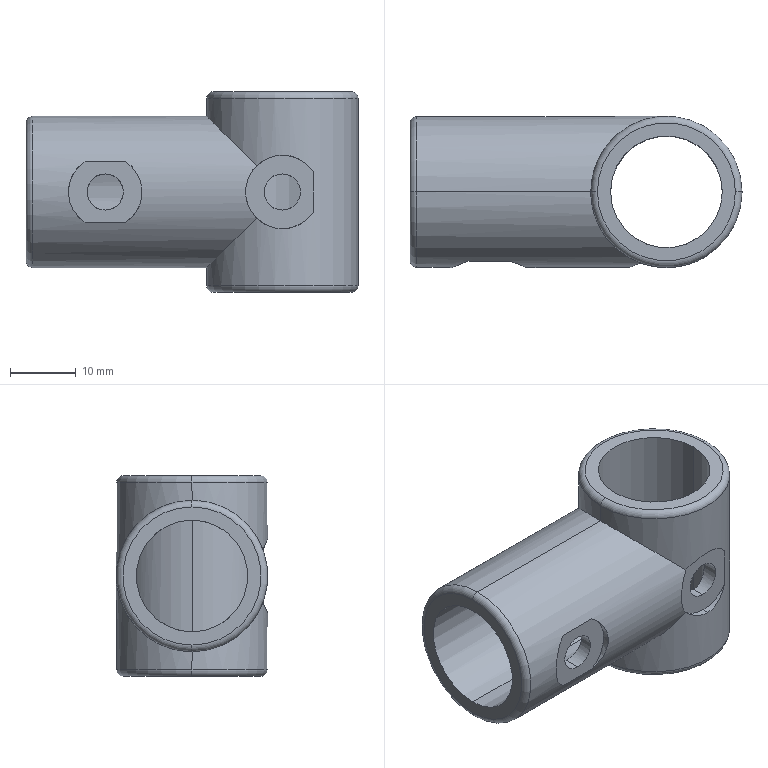Part | SolidWorks | features BaseBody 1 | 1 solid | 30 faces | box 50.5 x 23 x 30.5 mm | volume 11175 mm3 | cylinder 19 | torus 6 | plane 5 | commonest cylinder face diameters 23 x6 11.2 x5 5.5 x4 17 x4
STEP:
#1=CARTESIAN_POINT('',(0.,11.5,15.25));
#2=VERTEX_POINT('',#1);
#3=CARTESIAN_POINT('',(-11.5,0.,3.75));
#4=VERTEX_POINT('',#3);
#5=CARTESIAN_POINT('',(0.,11.5,15.25));
#6=CARTESIAN_POINT('',(-6.737,11.5,8.513));
#7=CARTESIAN_POINT('',(-11.5,6.737,3.75));
#8=CARTESIAN_POINT('',(-11.5,0.,3.75));
#9=(BOUNDED_CURVE()B_SPLINE_CURVE(3,(#5,#6,#7,#8),.UNSPECIFIED.,.F.,.F.)B_SPLINE_CURVE_WITH_KNOTS((4,4),(4.712,6.283),.UNSPECIFIED.)CURVE()GEOMETRIC_REPRESENTATION_ITEM()RATIONAL_B_SPLINE_CURVE((1.,0.8047,0.8047,1.))REPRESENTATION_ITEM(''));
#10=EDGE_CURVE('',#2,#4,#9,.T.);
#11=ORIENTED_EDGE('',*,*,#10,.T.);
#12=CARTESIAN_POINT('',(-38.,0.,3.75));
#13=VERTEX_POINT('',#12);
#14=CARTESIAN_POINT('',(11.501,0.,3.75));
#15=DIRECTION('',(-1.,0.,0.));
#16=VECTOR('',#15,1000.);
#17=LINE('',#14,#16);
#18=EDGE_CURVE('',#4,#13,#17,.T.);
#19=ORIENTED_EDGE('',*,*,#18,.T.);
#20=CARTESIAN_POINT('',(-38.,0.,26.75));
#21=VERTEX_POINT('',#20);
#22=CARTESIAN_POINT('',(-38.,0.,15.25));
#23=DIRECTION('',(1.,0.,0.));
#24=DIRECTION('',(0.,0.,1.));
#25=AXIS2_PLACEMENT_3D('',#22,#23,#24);
#26=CIRCLE('',#25,11.5);
#27=EDGE_CURVE('',#13,#21,#26,.T.);
#28=ORIENTED_EDGE('',*,*,#27,.T.);
#29=CARTESIAN_POINT('',(-11.5,0.,26.75));
#30=VERTEX_POINT('',#29);
#31=CARTESIAN_POINT('',(11.501,0.,26.75));
#32=DIRECTION('',(-1.,0.,0.));
#33=VECTOR('',#32,1000.);
#34=LINE('',#31,#33);
#35=EDGE_CURVE('',#30,#21,#34,.T.);
#36=ORIENTED_EDGE('',*,*,#35,.F.);
#37=CARTESIAN_POINT('',(-11.5,0.,26.75));
#38=CARTESIAN_POINT('',(-11.5,6.737,26.75));
#39=CARTESIAN_POINT('',(-6.737,11.5,21.987));
#40=CARTESIAN_POINT('',(0.,11.5,15.25));
#41=(BOUNDED_CURVE()B_SPLINE_CURVE(3,(#37,#38,#39,#40),.UNSPECIFIED.,.F.,.F.)B_SPLINE_CURVE_WITH_KNOTS((4,4),(3.142,4.712),.UNSPECIFIED.)CURVE()GEOMETRIC_REPRESENTATION_ITEM()RATIONAL_B_SPLINE_CURVE((1.,0.8047,0.8047,1.))REPRESENTATION_ITEM(''));
#42=EDGE_CURVE('',#30,#2,#41,.T.);
#43=ORIENTED_EDGE('',*,*,#42,.T.);
#44=EDGE_LOOP('',(#11,#19,#28,#36,#43));
#45=FACE_OUTER_BOUND('',#44,.T.);
#46=CARTESIAN_POINT('',(11.501,0.,15.25));
#47=DIRECTION('',(-1.,0.,0.));
#48=DIRECTION('',(0.,0.,1.));
#49=AXIS2_PLACEMENT_3D('',#46,#47,#48);
#50=CYLINDRICAL_SURFACE('',#49,11.5);
#51=ADVANCED_FACE('',(#45),#50,.T.);
#52=CARTESIAN_POINT('',(-11.5,0.,29.5));
#53=VERTEX_POINT('',#52);
#54=CARTESIAN_POINT('',(11.5,0.,29.5));
#55=VERTEX_POINT('',#54);
#56=CARTESIAN_POINT('',(0.,0.,29.5));
#57=DIRECTION('',(0.,0.,-1.));
#58=DIRECTION('',(-1.,0.,0.));
#59=AXIS2_PLACEMENT_3D('',#56,#57,#58);
#60=CIRCLE('',#59,11.5);
#61=EDGE_CURVE('',#53,#55,#60,.T.);
#62=ORIENTED_EDGE('',*,*,#61,.T.);
#63=CARTESIAN_POINT('',(11.5,0.,1.));
#64=VERTEX_POINT('',#63);
#65=CARTESIAN_POINT('',(11.5,0.,30.5));
#66=DIRECTION('',(0.,0.,-1.));
#67=VECTOR('',#66,1000.);
#68=LINE('',#65,#67);
#69=EDGE_CURVE('',#55,#64,#68,.T.);
#70=ORIENTED_EDGE('',*,*,#69,.T.);
#71=CARTESIAN_POINT('',(-11.5,0.,1.));
#72=VERTEX_POINT('',#71);
#73=CARTESIAN_POINT('',(0.,0.,1.));
#74=DIRECTION('',(0.,0.,1.));
#75=DIRECTION('',(-1.,0.,0.));
#76=AXIS2_PLACEMENT_3D('',#73,#74,#75);
#77=CIRCLE('',#76,11.5);
#78=EDGE_CURVE('',#64,#72,#77,.T.);
#79=ORIENTED_EDGE('',*,*,#78,.T.);
#80=CARTESIAN_POINT('',(-11.5,0.,30.5));
#81=DIRECTION('',(0.,0.,-1.));
#82=VECTOR('',#81,1000.);
#83=LINE('',#80,#82);
#84=EDGE_CURVE('',#4,#72,#83,.T.);
#85=ORIENTED_EDGE('',*,*,#84,.F.);
#86=ORIENTED_EDGE('',*,*,#10,.F.);
#87=ORIENTED_EDGE('',*,*,#42,.F.);
#88=CARTESIAN_POINT('',(-11.5,0.,30.5));
#89=DIRECTION('',(0.,0.,-1.));
#90=VECTOR('',#89,1000.);
#91=LINE('',#88,#90);
#92=EDGE_CURVE('',#53,#30,#91,.T.);
#93=ORIENTED_EDGE('',*,*,#92,.F.);
#94=EDGE_LOOP('',(#62,#70,#79,#85,#86,#87,#93));
#95=FACE_OUTER_BOUND('',#94,.T.);
#96=CARTESIAN_POINT('',(0.,0.,30.5));
#97=DIRECTION('',(0.,0.,-1.));
#98=DIRECTION('',(-1.,0.,0.));
#99=AXIS2_PLACEMENT_3D('',#96,#97,#98);
#100=CYLINDRICAL_SURFACE('',#99,11.5);
#101=ADVANCED_FACE('',(#95),#100,.T.);
#102=CARTESIAN_POINT('',(-39.,0.,4.75));
#103=VERTEX_POINT('',#102);
#104=CARTESIAN_POINT('',(-39.,0.,25.75));
#105=VERTEX_POINT('',#104);
#106=CARTESIAN_POINT('',(-39.,0.,15.25));
#107=DIRECTION('',(1.,0.,0.));
#108=DIRECTION('',(0.,0.,-1.));
#109=AXIS2_PLACEMENT_3D('',#106,#107,#108);
#110=CIRCLE('',#109,10.5);
#111=EDGE_CURVE('',#103,#105,#110,.T.);
#112=ORIENTED_EDGE('',*,*,#111,.T.);
#113=CARTESIAN_POINT('',(-38.,0.,25.75));
#114=DIRECTION('',(0.,1.,0.));
#115=DIRECTION('',(0.,0.,1.));
#116=AXIS2_PLACEMENT_3D('',#113,#114,#115);
#117=CIRCLE('',#116,1.);
#118=EDGE_CURVE('',#105,#21,#117,.T.);
#119=ORIENTED_EDGE('',*,*,#118,.T.);
#120=ORIENTED_EDGE('',*,*,#27,.F.);
#121=CARTESIAN_POINT('',(-38.,0.,4.75));
#122=DIRECTION('',(0.,-1.,0.));
#123=DIRECTION('',(0.,0.,-1.));
#124=AXIS2_PLACEMENT_3D('',#121,#122,#123);
#125=CIRCLE('',#124,1.);
#126=EDGE_CURVE('',#103,#13,#125,.T.);
#127=ORIENTED_EDGE('',*,*,#126,.F.);
#128=EDGE_LOOP('',(#112,#119,#120,#127));
#129=FACE_OUTER_BOUND('',#128,.T.);
#130=CARTESIAN_POINT('',(-38.,0.,15.25));
#131=DIRECTION('',(1.,0.,0.));
#132=DIRECTION('',(0.,0.,-1.));
#133=AXIS2_PLACEMENT_3D('',#130,#131,#132);
#134=TOROIDAL_SURFACE('',#133,10.5,1.);
#135=ADVANCED_FACE('',(#129),#134,.T.);
#136=CARTESIAN_POINT('',(10.5,0.,0.));
#137=VERTEX_POINT('',#136);
#138=CARTESIAN_POINT('',(-10.5,0.,0.));
#139=VERTEX_POINT('',#138);
#140=CARTESIAN_POINT('',(0.,0.,0.));
#141=DIRECTION('',(0.,0.,1.));
#142=DIRECTION('',(1.,0.,0.));
#143=AXIS2_PLACEMENT_3D('',#140,#141,#142);
#144=CIRCLE('',#143,10.5);
#145=EDGE_CURVE('',#137,#139,#144,.T.);
#146=ORIENTED_EDGE('',*,*,#145,.T.);
#147=CARTESIAN_POINT('',(-10.5,0.,1.));
#148=DIRECTION('',(0.,1.,0.));
#149=DIRECTION('',(-1.,0.,0.));
#150=AXIS2_PLACEMENT_3D('',#147,#148,#149);
#151=CIRCLE('',#150,1.);
#152=EDGE_CURVE('',#139,#72,#151,.T.);
#153=ORIENTED_EDGE('',*,*,#152,.T.);
#154=ORIENTED_EDGE('',*,*,#78,.F.);
#155=CARTESIAN_POINT('',(10.5,0.,1.));
#156=DIRECTION('',(0.,-1.,0.));
#157=DIRECTION('',(0.,0.,-1.));
#158=AXIS2_PLACEMENT_3D('',#155,#156,#157);
#159=CIRCLE('',#158,1.);
#160=EDGE_CURVE('',#137,#64,#159,.T.);
#161=ORIENTED_EDGE('',*,*,#160,.F.);
#162=EDGE_LOOP('',(#146,#153,#154,#161));
#163=FACE_OUTER_BOUND('',#162,.T.);
#164=CARTESIAN_POINT('',(0.,0.,1.));
#165=DIRECTION('',(0.,0.,1.));
#166=DIRECTION('',(1.,0.,0.));
#167=AXIS2_PLACEMENT_3D('',#164,#165,#166);
#168=TOROIDAL_SURFACE('',#167,10.5,1.);
#169=ADVANCED_FACE('',(#163),#168,.T.);
#170=ORIENTED_EDGE('',*,*,#61,.F.);
#171=CARTESIAN_POINT('',(-10.5,0.,30.5));
#172=VERTEX_POINT('',#171);
#173=CARTESIAN_POINT('',(-10.5,0.,29.5));
#174=DIRECTION('',(0.,1.,0.));
#175=DIRECTION('',(-1.,0.,0.));
#176=AXIS2_PLACEMENT_3D('',#173,#174,#175);
#177=CIRCLE('',#176,1.);
#178=EDGE_CURVE('',#53,#172,#177,.T.);
#179=ORIENTED_EDGE('',*,*,#178,.T.);
#180=CARTESIAN_POINT('',(10.5,0.,30.5));
#181=VERTEX_POINT('',#180);
#182=CARTESIAN_POINT('',(0.,0.,30.5));
#183=DIRECTION('',(0.,0.,-1.));
#184=DIRECTION('',(1.,0.,0.));
#185=AXIS2_PLACEMENT_3D('',#182,#183,#184);
#186=CIRCLE('',#185,10.5);
#187=EDGE_CURVE('',#172,#181,#186,.T.);
#188=ORIENTED_EDGE('',*,*,#187,.T.);
#189=CARTESIAN_POINT('',(10.5,0.,29.5));
#190=DIRECTION('',(0.,-1.,0.));
#191=DIRECTION('',(0.,0.,-1.));
#192=AXIS2_PLACEMENT_3D('',#189,#190,#191);
#193=CIRCLE('',#192,1.);
#194=EDGE_CURVE('',#55,#181,#193,.T.);
#195=ORIENTED_EDGE('',*,*,#194,.F.);
#196=EDGE_LOOP('',(#170,#179,#188,#195));
#197=FACE_OUTER_BOUND('',#196,.T.);
#198=CARTESIAN_POINT('',(0.,0.,29.5));
#199=DIRECTION('',(0.,0.,1.));
#200=DIRECTION('',(1.,0.,0.));
#201=AXIS2_PLACEMENT_3D('',#198,#199,#200);
#202=TOROIDAL_SURFACE('',#201,10.5,1.);
#203=ADVANCED_FACE('',(#197),#202,.T.);
#204=CARTESIAN_POINT('',(0.,-10.5,20.85));
#205=VERTEX_POINT('',#204);
#206=CARTESIAN_POINT('',(0.,-10.5,9.65));
#207=VERTEX_POINT('',#206);
#208=CARTESIAN_POINT('',(0.,-10.5,15.25));
#209=DIRECTION('',(0.,-1.,0.));
#210=DIRECTION('',(0.,0.,-1.));
#211=AXIS2_PLACEMENT_3D('',#208,#209,#210);
#212=CIRCLE('',#211,5.6);
#213=EDGE_CURVE('',#205,#207,#212,.T.);
#214=ORIENTED_EDGE('',*,*,#213,.F.);
#215=CARTESIAN_POINT('',(0.,-11.5,20.85));
#216=VERTEX_POINT('',#215);
#217=CARTESIAN_POINT('',(0.,-10.5,20.85));
#218=DIRECTION('',(0.,-1.,0.));
#219=VECTOR('',#218,1000.);
#220=LINE('',#217,#219);
#221=EDGE_CURVE('',#205,#216,#220,.T.);
#222=ORIENTED_EDGE('',*,*,#221,.T.);
#223=CARTESIAN_POINT('',(-3.96,-10.797,19.21));
#224=VERTEX_POINT('',#223);
#225=CARTESIAN_POINT('',(-3.96,-10.797,19.21));
#226=CARTESIAN_POINT('',(-3.703,-10.891,19.467));
#227=CARTESIAN_POINT('',(-3.425,-10.983,19.695));
#228=CARTESIAN_POINT('',(-2.976,-11.109,19.997));
#229=CARTESIAN_POINT('',(-2.821,-11.15,20.091));
#230=CARTESIAN_POINT('',(-2.5,-11.226,20.264));
#231=CARTESIAN_POINT('',(-2.333,-11.262,20.344));
#232=CARTESIAN_POINT('',(-1.826,-11.359,20.557));
#233=CARTESIAN_POINT('',(-1.476,-11.411,20.665));
#234=CARTESIAN_POINT('',(-0.7521,-11.481,20.812));
#235=CARTESIAN_POINT('',(-0.3759,-11.5,20.85));
#236=CARTESIAN_POINT('',(0.,-11.5,20.85));
#237=B_SPLINE_CURVE_WITH_KNOTS('',3,(#225,#226,#227,#228,#229,#230,#231,#232,#233,#234,#235,#236),.UNSPECIFIED.,.F.,.F.,(4,2,2,2,2,4),(-0.004442,-0.003332,-0.002776,-0.002221,-0.001111,0.),.UNSPECIFIED.);
#238=EDGE_CURVE('',#224,#216,#237,.T.);
#239=ORIENTED_EDGE('',*,*,#238,.F.);
#240=CARTESIAN_POINT('',(-3.96,-10.797,11.29));
#241=VERTEX_POINT('',#240);
#242=CARTESIAN_POINT('',(-3.96,-10.797,11.29));
#243=CARTESIAN_POINT('',(-4.217,-10.891,11.547));
#244=CARTESIAN_POINT('',(-4.445,-10.983,11.825));
#245=CARTESIAN_POINT('',(-4.747,-11.109,12.274));
#246=CARTESIAN_POINT('',(-4.841,-11.15,12.429));
#247=CARTESIAN_POINT('',(-5.015,-11.226,12.751));
#248=CARTESIAN_POINT('',(-5.094,-11.262,12.918));
#249=CARTESIAN_POINT('',(-5.307,-11.359,13.425));
#250=CARTESIAN_POINT('',(-5.415,-11.411,13.775));
#251=CARTESIAN_POINT('',(-5.562,-11.481,14.499));
#252=CARTESIAN_POINT('',(-5.6,-11.5,14.876));
#253=CARTESIAN_POINT('',(-5.6,-11.5,15.617));
#254=CARTESIAN_POINT('',(-5.564,-11.482,15.986));
#255=CARTESIAN_POINT('',(-5.417,-11.412,16.719));
#256=CARTESIAN_POINT('',(-5.308,-11.36,17.071));
#257=CARTESIAN_POINT('',(-5.026,-11.231,17.746));
#258=CARTESIAN_POINT('',(-4.85,-11.153,18.072));
#259=CARTESIAN_POINT('',(-4.446,-10.983,18.674));
#260=CARTESIAN_POINT('',(-4.217,-10.891,18.953));
#261=CARTESIAN_POINT('',(-3.96,-10.797,19.21));
#262=B_SPLINE_CURVE_WITH_KNOTS('',3,(#242,#243,#244,#245,#246,#247,#248,#249,#250,#251,#252,#253,#254,#255,#256,#257,#258,#259,#260,#261),.UNSPECIFIED.,.F.,.F.,(4,2,2,2,2,2,2,2,2,4),(0.,0.001111,0.001667,0.002222,0.003334,0.004445,0.005556,0.006667,0.007779,0.00889),.UNSPECIFIED.);
#263=EDGE_CURVE('',#241,#224,#262,.T.);
#264=ORIENTED_EDGE('',*,*,#263,.F.);
#265=CARTESIAN_POINT('',(0.,-11.5,9.65));
#266=VERTEX_POINT('',#265);
#267=CARTESIAN_POINT('',(0.,-11.5,9.65));
#268=CARTESIAN_POINT('',(-0.3755,-11.5,9.65));
#269=CARTESIAN_POINT('',(-0.7436,-11.482,9.687));
#270=CARTESIAN_POINT('',(-1.466,-11.412,9.833));
#271=CARTESIAN_POINT('',(-1.824,-11.36,9.943));
#272=CARTESIAN_POINT('',(-2.499,-11.23,10.225));
#273=CARTESIAN_POINT('',(-2.818,-11.154,10.397));
#274=CARTESIAN_POINT('',(-3.422,-10.984,10.802));
#275=CARTESIAN_POINT('',(-3.703,-10.891,11.034));
#276=CARTESIAN_POINT('',(-3.96,-10.797,11.29));
#277=B_SPLINE_CURVE_WITH_KNOTS('',3,(#267,#268,#269,#270,#271,#272,#273,#274,#275,#276),.UNSPECIFIED.,.F.,.F.,(4,2,2,2,4),(0.,0.001109,0.002219,0.003328,0.004437),.UNSPECIFIED.);
#278=EDGE_CURVE('',#266,#241,#277,.T.);
#279=ORIENTED_EDGE('',*,*,#278,.F.);
#280=CARTESIAN_POINT('',(0.,-10.5,9.65));
#281=DIRECTION('',(0.,-1.,0.));
#282=VECTOR('',#281,1000.);
#283=LINE('',#280,#282);
#284=EDGE_CURVE('',#207,#266,#283,.T.);
#285=ORIENTED_EDGE('',*,*,#284,.F.);
#286=EDGE_LOOP('',(#214,#222,#239,#264,#279,#285));
#287=FACE_OUTER_BOUND('',#286,.T.);
#288=CARTESIAN_POINT('',(0.,-10.5,15.25));
#289=DIRECTION('',(0.,-1.,0.));
#290=DIRECTION('',(0.,0.,-1.));
#291=AXIS2_PLACEMENT_3D('',#288,#289,#290);
#292=CYLINDRICAL_SURFACE('',#291,5.6);
#293=ADVANCED_FACE('',(#287),#292,.F.);
#294=CARTESIAN_POINT('',(4.69,-10.5,12.191));
#295=VERTEX_POINT('',#294);
#296=CARTESIAN_POINT('',(0.,-10.5,15.25));
#297=DIRECTION('',(0.,-1.,0.));
#298=DIRECTION('',(0.,0.,-1.));
#299=AXIS2_PLACEMENT_3D('',#296,#297,#298);
#300=CIRCLE('',#299,5.6);
#301=EDGE_CURVE('',#207,#295,#300,.T.);
#302=ORIENTED_EDGE('',*,*,#301,.F.);
#303=ORIENTED_EDGE('',*,*,#284,.T.);
#304=CARTESIAN_POINT('',(4.69,-10.5,12.191));
#305=CARTESIAN_POINT('',(4.437,-10.613,11.803));
#306=CARTESIAN_POINT('',(4.144,-10.733,11.456));
#307=CARTESIAN_POINT('',(3.642,-10.909,10.99));
#308=CARTESIAN_POINT('',(3.464,-10.968,10.844));
#309=CARTESIAN_POINT('',(3.089,-11.079,10.574));
#310=CARTESIAN_POINT('',(2.895,-11.132,10.451));
#311=CARTESIAN_POINT('',(2.493,-11.229,10.23));
#312=CARTESIAN_POINT('',(2.284,-11.273,10.132));
#313=CARTESIAN_POINT('',(1.852,-11.352,9.96));
#314=CARTESIAN_POINT('',(1.627,-11.387,9.886));
#315=CARTESIAN_POINT('',(0.9434,-11.47,9.71));
#316=CARTESIAN_POINT('',(0.4773,-11.5,9.65));
#317=CARTESIAN_POINT('',(0.,-11.5,9.65));
#318=B_SPLINE_CURVE_WITH_KNOTS('',3,(#304,#305,#306,#307,#308,#309,#310,#311,#312,#313,#314,#315,#316,#317),.UNSPECIFIED.,.F.,.F.,(4,2,2,2,2,2,4),(-0.005641,-0.00423,-0.003525,-0.00282,-0.002115,-0.00141,0.),.UNSPECIFIED.);
#319=EDGE_CURVE('',#295,#266,#318,.T.);
#320=ORIENTED_EDGE('',*,*,#319,.F.);
#321=EDGE_LOOP('',(#302,#303,#320));
#322=FACE_OUTER_BOUND('',#321,.T.);
#323=CARTESIAN_POINT('',(0.,-10.5,15.25));
#324=DIRECTION('',(0.,-1.,0.));
#325=DIRECTION('',(0.,0.,-1.));
#326=AXIS2_PLACEMENT_3D('',#323,#324,#325);
#327=CYLINDRICAL_SURFACE('',#326,5.6);
#328=ADVANCED_FACE('',(#322),#327,.F.);
#329=CARTESIAN_POINT('',(-26.95,-10.5,18.));
#330=VERTEX_POINT('',#329);
#331=CARTESIAN_POINT('',(-26.95,-10.5,12.5));
#332=VERTEX_POINT('',#331);
#333=CARTESIAN_POINT('',(-26.95,-10.5,15.25));
#334=DIRECTION('',(0.,-1.,0.));
#335=DIRECTION('',(0.,0.,1.));
#336=AXIS2_PLACEMENT_3D('',#333,#334,#335);
#337=CIRCLE('',#336,2.75);
#338=EDGE_CURVE('',#330,#332,#337,.T.);
#339=ORIENTED_EDGE('',*,*,#338,.T.);
#340=CARTESIAN_POINT('',(-26.95,-8.043,12.5));
#341=VERTEX_POINT('',#340);
#342=CARTESIAN_POINT('',(-26.95,-11.5,12.5));
#343=DIRECTION('',(0.,1.,0.));
#344=VECTOR('',#343,1000.);
#345=LINE('',#342,#344);
#346=EDGE_CURVE('',#332,#341,#345,.T.);
#347=ORIENTED_EDGE('',*,*,#346,.T.);
#348=CARTESIAN_POINT('',(-26.95,-8.043,18.));
#349=VERTEX_POINT('',#348);
#350=CARTESIAN_POINT('',(-26.95,-8.043,18.));
#351=CARTESIAN_POINT('',(-27.133,-8.043,18.));
#352=CARTESIAN_POINT('',(-27.313,-8.049,17.982));
#353=CARTESIAN_POINT('',(-27.666,-8.073,17.911));
#354=CARTESIAN_POINT('',(-27.841,-8.09,17.858));
#355=CARTESIAN_POINT('',(-28.173,-8.134,17.72));
#356=CARTESIAN_POINT('',(-28.331,-8.159,17.635));
#357=CARTESIAN_POINT('',(-28.628,-8.215,17.436));
#358=CARTESIAN_POINT('',(-28.768,-8.245,17.321));
#359=CARTESIAN_POINT('',(-29.146,-8.334,16.943));
#360=CARTESIAN_POINT('',(-29.351,-8.392,16.638));
#361=CARTESIAN_POINT('',(-29.557,-8.455,16.143));
#362=CARTESIAN_POINT('',(-29.611,-8.471,15.968));
#363=CARTESIAN_POINT('',(-29.682,-8.494,15.613));
#364=CARTESIAN_POINT('',(-29.7,-8.5,15.434));
#365=CARTESIAN_POINT('',(-29.7,-8.5,15.072));
#366=CARTESIAN_POINT('',(-29.682,-8.494,14.889));
#367=CARTESIAN_POINT('',(-29.612,-8.472,14.535));
#368=CARTESIAN_POINT('',(-29.559,-8.455,14.363));
#369=CARTESIAN_POINT('',(-29.42,-8.413,14.028));
#370=CARTESIAN_POINT('',(-29.335,-8.388,13.869));
#371=CARTESIAN_POINT('',(-29.136,-8.334,13.573));
#372=CARTESIAN_POINT('',(-29.022,-8.304,13.433));
#373=CARTESIAN_POINT('',(-28.768,-8.245,13.179));
#374=CARTESIAN_POINT('',(-28.631,-8.215,13.066));
#375=CARTESIAN_POINT('',(-28.334,-8.16,12.867));
#376=CARTESIAN_POINT('',(-28.174,-8.134,12.781));
#377=CARTESIAN_POINT('',(-27.843,-8.091,12.643));
#378=CARTESIAN_POINT('',(-27.671,-8.073,12.59));
#379=CARTESIAN_POINT('',(-27.316,-8.049,12.518));
#380=CARTESIAN_POINT('',(-27.133,-8.043,12.5));
#381=CARTESIAN_POINT('',(-26.95,-8.043,12.5));
#382=B_SPLINE_CURVE_WITH_KNOTS('',3,(#350,#351,#352,#353,#354,#355,#356,#357,#358,#359,#360,#361,#362,#363,#364,#365,#366,#367,#368,#369,#370,#371,#372,#373,#374,#375,#376,#377,#378,#379,#380,#381),.UNSPECIFIED.,.F.,.F.,(4,2,2,2,2,2,2,2,2,2,2,2,2,2,2,4),(0.,0.0005408,0.001082,0.001622,0.002163,0.003245,0.003786,0.004326,0.004867,0.005408,0.005949,0.00649,0.007031,0.007571,0.008112,0.008653),.UNSPECIFIED.);
#383=EDGE_CURVE('',#349,#341,#382,.T.);
#384=ORIENTED_EDGE('',*,*,#383,.F.);
#385=CARTESIAN_POINT('',(-26.95,-11.5,18.));
#386=DIRECTION('',(0.,1.,0.));
#387=VECTOR('',#386,1000.);
#388=LINE('',#385,#387);
#389=EDGE_CURVE('',#330,#349,#388,.T.);
#390=ORIENTED_EDGE('',*,*,#389,.F.);
#391=EDGE_LOOP('',(#339,#347,#384,#390));
#392=FACE_OUTER_BOUND('',#391,.T.);
#393=CARTESIAN_POINT('',(-26.95,-11.5,15.25));
#394=DIRECTION('',(0.,1.,0.));
#395=DIRECTION('',(0.,0.,1.));
#396=AXIS2_PLACEMENT_3D('',#393,#394,#395);
#397=CYLINDRICAL_SURFACE('',#396,2.75);
#398=ADVANCED_FACE('',(#392),#397,.F.);
#399=ORIENTED_EDGE('',*,*,#383,.T.);
#400=CARTESIAN_POINT('',(-26.95,-8.043,12.5));
#401=CARTESIAN_POINT('',(-26.767,-8.043,12.5));
#402=CARTESIAN_POINT('',(-26.587,-8.049,12.518));
#403=CARTESIAN_POINT('',(-26.234,-8.073,12.589));
#404=CARTESIAN_POINT('',(-26.059,-8.09,12.642));
#405=CARTESIAN_POINT('',(-25.727,-8.134,12.78));
#406=CARTESIAN_POINT('',(-25.569,-8.159,12.865));
#407=CARTESIAN_POINT('',(-25.272,-8.215,13.064));
#408=CARTESIAN_POINT('',(-25.132,-8.245,13.179));
#409=CARTESIAN_POINT('',(-24.754,-8.334,13.557));
#410=CARTESIAN_POINT('',(-24.549,-8.392,13.862));
#411=CARTESIAN_POINT('',(-24.343,-8.455,14.357));
#412=CARTESIAN_POINT('',(-24.289,-8.471,14.532));
#413=CARTESIAN_POINT('',(-24.218,-8.494,14.887));
#414=CARTESIAN_POINT('',(-24.2,-8.5,15.066));
#415=CARTESIAN_POINT('',(-24.2,-8.5,15.428));
#416=CARTESIAN_POINT('',(-24.218,-8.494,15.611));
#417=CARTESIAN_POINT('',(-24.288,-8.472,15.965));
#418=CARTESIAN_POINT('',(-24.341,-8.455,16.137));
#419=CARTESIAN_POINT('',(-24.48,-8.413,16.472));
#420=CARTESIAN_POINT('',(-24.565,-8.388,16.631));
#421=CARTESIAN_POINT('',(-24.764,-8.334,16.927));
#422=CARTESIAN_POINT('',(-24.878,-8.304,17.067));
#423=CARTESIAN_POINT('',(-25.132,-8.245,17.321));
#424=CARTESIAN_POINT('',(-25.269,-8.215,17.434));
#425=CARTESIAN_POINT('',(-25.566,-8.16,17.633));
#426=CARTESIAN_POINT('',(-25.726,-8.134,17.719));
#427=CARTESIAN_POINT('',(-26.057,-8.091,17.857));
#428=CARTESIAN_POINT('',(-26.229,-8.073,17.91));
#429=CARTESIAN_POINT('',(-26.584,-8.049,17.982));
#430=CARTESIAN_POINT('',(-26.767,-8.043,18.));
#431=CARTESIAN_POINT('',(-26.95,-8.043,18.));
#432=B_SPLINE_CURVE_WITH_KNOTS('',3,(#400,#401,#402,#403,#404,#405,#406,#407,#408,#409,#410,#411,#412,#413,#414,#415,#416,#417,#418,#419,#420,#421,#422,#423,#424,#425,#426,#427,#428,#429,#430,#431),.UNSPECIFIED.,.F.,.F.,(4,2,2,2,2,2,2,2,2,2,2,2,2,2,2,4),(0.008653,0.009194,0.009734,0.01028,0.01082,0.0119,0.01244,0.01298,0.01352,0.01406,0.0146,0.01514,0.01568,0.01622,0.01676,0.01731),.UNSPECIFIED.);
#433=EDGE_CURVE('',#341,#349,#432,.T.);
#434=ORIENTED_EDGE('',*,*,#433,.T.);
#435=EDGE_LOOP('',(#399,#434));
#436=FACE_BOUND('',#435,.T.);
#437=CARTESIAN_POINT('',(-11.5,0.,6.75));
#438=VERTEX_POINT('',#437);
#439=CARTESIAN_POINT('',(-11.5,0.,23.75));
#440=VERTEX_POINT('',#439);
#441=CARTESIAN_POINT('',(-11.5,0.,6.75));
#442=CARTESIAN_POINT('',(-11.5,-0.5885,6.75));
#443=CARTESIAN_POINT('',(-11.455,-1.163,6.81));
#444=CARTESIAN_POINT('',(-11.327,-2.006,6.985));
#445=CARTESIAN_POINT('',(-11.274,-2.286,7.058));
#446=CARTESIAN_POINT('',(-11.149,-2.832,7.231));
#447=CARTESIAN_POINT('',(-11.078,-3.097,7.329));
#448=CARTESIAN_POINT('',(-10.922,-3.611,7.55));
#449=CARTESIAN_POINT('',(-10.836,-3.86,7.672));
#450=CARTESIAN_POINT('',(-10.651,-4.344,7.938));
#451=CARTESIAN_POINT('',(-10.552,-4.579,8.084));
#452=CARTESIAN_POINT('',(-10.241,-5.256,8.548));
#453=CARTESIAN_POINT('',(-10.017,-5.667,8.892));
#454=CARTESIAN_POINT('',(-9.553,-6.418,9.652));
#455=CARTESIAN_POINT('',(-9.312,-6.759,10.068));
#456=CARTESIAN_POINT('',(-8.851,-7.352,10.952));
#457=CARTESIAN_POINT('',(-8.628,-7.608,11.421));
#458=CARTESIAN_POINT('',(-8.33,-7.93,12.177));
#459=CARTESIAN_POINT('',(-8.236,-8.027,12.439));
#460=CARTESIAN_POINT('',(-8.069,-8.194,12.974));
#461=CARTESIAN_POINT('',(-7.996,-8.265,13.246));
#462=CARTESIAN_POINT('',(-7.875,-8.381,13.803));
#463=CARTESIAN_POINT('',(-7.827,-8.425,14.088));
#464=CARTESIAN_POINT('',(-7.762,-8.485,14.67));
#465=CARTESIAN_POINT('',(-7.746,-8.5,14.961));
#466=CARTESIAN_POINT('',(-7.746,-8.5,15.541));
#467=CARTESIAN_POINT('',(-7.762,-8.485,15.83));
#468=CARTESIAN_POINT('',(-7.827,-8.426,16.406));
#469=CARTESIAN_POINT('',(-7.875,-8.381,16.695));
#470=CARTESIAN_POINT('',(-8.057,-8.207,17.534));
#471=CARTESIAN_POINT('',(-8.228,-8.04,18.063));
#472=CARTESIAN_POINT('',(-8.527,-7.718,18.823));
#473=CARTESIAN_POINT('',(-8.634,-7.598,19.07));
#474=CARTESIAN_POINT('',(-8.854,-7.341,19.543));
#475=CARTESIAN_POINT('',(-8.967,-7.203,19.771));
#476=CARTESIAN_POINT('',(-9.312,-6.758,20.432));
#477=CARTESIAN_POINT('',(-9.549,-6.423,20.843));
#478=CARTESIAN_POINT('',(-10.017,-5.667,21.608));
#479=CARTESIAN_POINT('',(-10.24,-5.256,21.952));
#480=CARTESIAN_POINT('',(-10.548,-4.588,22.41));
#481=CARTESIAN_POINT('',(-10.646,-4.357,22.554));
#482=CARTESIAN_POINT('',(-10.83,-3.875,22.82));
#483=CARTESIAN_POINT('',(-10.918,-3.624,22.944));
#484=CARTESIAN_POINT('',(-11.155,-2.846,23.279));
#485=CARTESIAN_POINT('',(-11.281,-2.306,23.452));
#486=CARTESIAN_POINT('',(-11.411,-1.46,23.629));
#487=CARTESIAN_POINT('',(-11.444,-1.17,23.674));
#488=CARTESIAN_POINT('',(-11.489,-0.5874,23.735));
#489=CARTESIAN_POINT('',(-11.5,-0.294,23.75));
#490=CARTESIAN_POINT('',(-11.5,0.,23.75));
#491=B_SPLINE_CURVE_WITH_KNOTS('',3,(#441,#442,#443,#444,#445,#446,#447,#448,#449,#450,#451,#452,#453,#454,#455,#456,#457,#458,#459,#460,#461,#462,#463,#464,#465,#466,#467,#468,#469,#470,#471,#472,#473,#474,#475,#476,#477,#478,#479,#480,#481,#482,#483,#484,#485,#486,#487,#488,#489,#490),.UNSPECIFIED.,.F.,.F.,(4,2,2,2,2,2,2,2,2,2,2,2,2,2,2,2,2,2,2,2,2,2,2,2,4),(0.02779,0.02952,0.03039,0.03126,0.03213,0.03299,0.03473,0.03647,0.0382,0.03907,0.03994,0.0408,0.04167,0.04254,0.04341,0.04514,0.04601,0.04688,0.04861,0.05035,0.05122,0.05208,0.05382,0.05469,0.05555),.UNSPECIFIED.);
#492=EDGE_CURVE('',#438,#440,#491,.T.);
#493=ORIENTED_EDGE('',*,*,#492,.F.);
#494=CARTESIAN_POINT('',(-39.,0.,6.75));
#495=VERTEX_POINT('',#494);
#496=CARTESIAN_POINT('',(11.501,0.,6.75));
#497=DIRECTION('',(-1.,0.,0.));
#498=VECTOR('',#497,1000.);
#499=LINE('',#496,#498);
#500=EDGE_CURVE('',#438,#495,#499,.T.);
#501=ORIENTED_EDGE('',*,*,#500,.T.);
#502=CARTESIAN_POINT('',(-39.,0.,23.75));
#503=VERTEX_POINT('',#502);
#504=CARTESIAN_POINT('',(-39.,0.,15.25));
#505=DIRECTION('',(-1.,0.,0.));
#506=DIRECTION('',(0.,0.,1.));
#507=AXIS2_PLACEMENT_3D('',#504,#505,#506);
#508=CIRCLE('',#507,8.5);
#509=EDGE_CURVE('',#495,#503,#508,.T.);
#510=ORIENTED_EDGE('',*,*,#509,.T.);
#511=CARTESIAN_POINT('',(11.501,0.,23.75));
#512=DIRECTION('',(-1.,0.,0.));
#513=VECTOR('',#512,1000.);
#514=LINE('',#511,#513);
#515=EDGE_CURVE('',#440,#503,#514,.T.);
#516=ORIENTED_EDGE('',*,*,#515,.F.);
#517=EDGE_LOOP('',(#493,#501,#510,#516));
#518=FACE_OUTER_BOUND('',#517,.T.);
#519=CARTESIAN_POINT('',(11.501,0.,15.25));
#520=DIRECTION('',(-1.,0.,0.));
#521=DIRECTION('',(0.,0.,1.));
#522=AXIS2_PLACEMENT_3D('',#519,#520,#521);
#523=CYLINDRICAL_SURFACE('',#522,8.5);
#524=ADVANCED_FACE('',(#436,#518),#523,.F.);
#525=CARTESIAN_POINT('',(0.,-10.5,18.));
#526=VERTEX_POINT('',#525);
#527=CARTESIAN_POINT('',(0.,-10.5,12.5));
#528=VERTEX_POINT('',#527);
#529=CARTESIAN_POINT('',(0.,-10.5,15.25));
#530=DIRECTION('',(0.,-1.,0.));
#531=DIRECTION('',(0.,0.,1.));
#532=AXIS2_PLACEMENT_3D('',#529,#530,#531);
#533=CIRCLE('',#532,2.75);
#534=EDGE_CURVE('',#526,#528,#533,.T.);
#535=ORIENTED_EDGE('',*,*,#534,.T.);
#536=CARTESIAN_POINT('',(0.,-8.5,12.5));
#537=VERTEX_POINT('',#536);
#538=CARTESIAN_POINT('',(0.,-11.5,12.5));
#539=DIRECTION('',(0.,1.,0.));
#540=VECTOR('',#539,1000.);
#541=LINE('',#538,#540);
#542=EDGE_CURVE('',#528,#537,#541,.T.);
#543=ORIENTED_EDGE('',*,*,#542,.T.);
#544=CARTESIAN_POINT('',(0.,-8.5,18.));
#545=VERTEX_POINT('',#544);
#546=CARTESIAN_POINT('',(0.,-8.5,18.));
#547=CARTESIAN_POINT('',(-0.183,-8.5,18.));
#548=CARTESIAN_POINT('',(-0.3626,-8.494,17.982));
#549=CARTESIAN_POINT('',(-0.7157,-8.472,17.911));
#550=CARTESIAN_POINT('',(-0.891,-8.455,17.858));
#551=CARTESIAN_POINT('',(-1.223,-8.413,17.719));
#552=CARTESIAN_POINT('',(-1.381,-8.388,17.635));
#553=CARTESIAN_POINT('',(-1.679,-8.334,17.435));
#554=CARTESIAN_POINT('',(-1.819,-8.304,17.32));
#555=CARTESIAN_POINT('',(-2.197,-8.215,16.942));
#556=CARTESIAN_POINT('',(-2.401,-8.155,16.638));
#557=CARTESIAN_POINT('',(-2.607,-8.091,16.143));
#558=CARTESIAN_POINT('',(-2.661,-8.073,15.968));
#559=CARTESIAN_POINT('',(-2.732,-8.049,15.613));
#560=CARTESIAN_POINT('',(-2.75,-8.043,15.434));
#561=CARTESIAN_POINT('',(-2.75,-8.043,15.072));
#562=CARTESIAN_POINT('',(-2.732,-8.049,14.889));
#563=CARTESIAN_POINT('',(-2.662,-8.073,14.535));
#564=CARTESIAN_POINT('',(-2.609,-8.09,14.363));
#565=CARTESIAN_POINT('',(-2.47,-8.133,14.028));
#566=CARTESIAN_POINT('',(-2.385,-8.159,13.87));
#567=CARTESIAN_POINT('',(-2.187,-8.215,13.573));
#568=CARTESIAN_POINT('',(-2.072,-8.245,13.433));
#569=CARTESIAN_POINT('',(-1.819,-8.304,13.18));
#570=CARTESIAN_POINT('',(-1.682,-8.333,13.067));
#571=CARTESIAN_POINT('',(-1.385,-8.388,12.867));
#572=CARTESIAN_POINT('',(-1.224,-8.413,12.781));
#573=CARTESIAN_POINT('',(-0.8928,-8.455,12.643));
#574=CARTESIAN_POINT('',(-0.7213,-8.471,12.59));
#575=CARTESIAN_POINT('',(-0.3658,-8.494,12.518));
#576=CARTESIAN_POINT('',(-0.183,-8.5,12.5));
#577=CARTESIAN_POINT('',(0.,-8.5,12.5));
#578=B_SPLINE_CURVE_WITH_KNOTS('',3,(#546,#547,#548,#549,#550,#551,#552,#553,#554,#555,#556,#557,#558,#559,#560,#561,#562,#563,#564,#565,#566,#567,#568,#569,#570,#571,#572,#573,#574,#575,#576,#577),.UNSPECIFIED.,.F.,.F.,(4,2,2,2,2,2,2,2,2,2,2,2,2,2,2,4),(0.,0.0005408,0.001082,0.001622,0.002163,0.003245,0.003786,0.004327,0.004867,0.005408,0.005949,0.00649,0.007031,0.007572,0.008112,0.008653),.UNSPECIFIED.);
#579=EDGE_CURVE('',#545,#537,#578,.T.);
#580=ORIENTED_EDGE('',*,*,#579,.F.);
#581=CARTESIAN_POINT('',(0.,-11.5,18.));
#582=DIRECTION('',(0.,1.,0.));
#583=VECTOR('',#582,1000.);
#584=LINE('',#581,#583);
#585=EDGE_CURVE('',#526,#545,#584,.T.);
#586=ORIENTED_EDGE('',*,*,#585,.F.);
#587=EDGE_LOOP('',(#535,#543,#580,#586));
#588=FACE_OUTER_BOUND('',#587,.T.);
#589=CARTESIAN_POINT('',(0.,-11.5,15.25));
#590=DIRECTION('',(0.,1.,0.));
#591=DIRECTION('',(0.,0.,1.));
#592=AXIS2_PLACEMENT_3D('',#589,#590,#591);
#593=CYLINDRICAL_SURFACE('',#592,2.75);
#594=ADVANCED_FACE('',(#588),#593,.F.);
#595=ORIENTED_EDGE('',*,*,#579,.T.);
#596=CARTESIAN_POINT('',(0.,-8.5,12.5));
#597=CARTESIAN_POINT('',(0.183,-8.5,12.5));
#598=CARTESIAN_POINT('',(0.3626,-8.494,12.518));
#599=CARTESIAN_POINT('',(0.7157,-8.472,12.589));
#600=CARTESIAN_POINT('',(0.891,-8.455,12.642));
#601=CARTESIAN_POINT('',(1.223,-8.413,12.781));
#602=CARTESIAN_POINT('',(1.381,-8.388,12.865));
#603=CARTESIAN_POINT('',(1.679,-8.334,13.065));
#604=CARTESIAN_POINT('',(1.819,-8.304,13.18));
#605=CARTESIAN_POINT('',(2.197,-8.215,13.558));
#606=CARTESIAN_POINT('',(2.401,-8.155,13.862));
#607=CARTESIAN_POINT('',(2.607,-8.091,14.357));
#608=CARTESIAN_POINT('',(2.661,-8.073,14.532));
#609=CARTESIAN_POINT('',(2.732,-8.049,14.887));
#610=CARTESIAN_POINT('',(2.75,-8.043,15.066));
#611=CARTESIAN_POINT('',(2.75,-8.043,15.428));
#612=CARTESIAN_POINT('',(2.732,-8.049,15.611));
#613=CARTESIAN_POINT('',(2.662,-8.073,15.965));
#614=CARTESIAN_POINT('',(2.609,-8.09,16.137));
#615=CARTESIAN_POINT('',(2.47,-8.133,16.472));
#616=CARTESIAN_POINT('',(2.385,-8.159,16.63));
#617=CARTESIAN_POINT('',(2.187,-8.215,16.927));
#618=CARTESIAN_POINT('',(2.072,-8.245,17.067));
#619=CARTESIAN_POINT('',(1.819,-8.304,17.32));
#620=CARTESIAN_POINT('',(1.682,-8.333,17.433));
#621=CARTESIAN_POINT('',(1.385,-8.388,17.633));
#622=CARTESIAN_POINT('',(1.224,-8.413,17.719));
#623=CARTESIAN_POINT('',(0.8928,-8.455,17.857));
#624=CARTESIAN_POINT('',(0.7213,-8.471,17.91));
#625=CARTESIAN_POINT('',(0.3658,-8.494,17.982));
#626=CARTESIAN_POINT('',(0.1829,-8.5,18.));
#627=CARTESIAN_POINT('',(0.,-8.5,18.));
#628=B_SPLINE_CURVE_WITH_KNOTS('',3,(#596,#597,#598,#599,#600,#601,#602,#603,#604,#605,#606,#607,#608,#609,#610,#611,#612,#613,#614,#615,#616,#617,#618,#619,#620,#621,#622,#623,#624,#625,#626,#627),.UNSPECIFIED.,.F.,.F.,(4,2,2,2,2,2,2,2,2,2,2,2,2,2,2,4),(0.008653,0.009194,0.009735,0.01028,0.01082,0.0119,0.01244,0.01298,0.01352,0.01406,0.0146,0.01514,0.01568,0.01622,0.01676,0.01731),.UNSPECIFIED.);
#629=EDGE_CURVE('',#537,#545,#628,.T.);
#630=ORIENTED_EDGE('',*,*,#629,.T.);
#631=EDGE_LOOP('',(#595,#630));
#632=FACE_BOUND('',#631,.T.);
#633=CARTESIAN_POINT('',(8.5,0.,30.5));
#634=VERTEX_POINT('',#633);
#635=CARTESIAN_POINT('',(-8.5,0.,30.5));
#636=VERTEX_POINT('',#635);
#637=CARTESIAN_POINT('',(0.,0.,30.5));
#638=DIRECTION('',(0.,0.,-1.));
#639=DIRECTION('',(-1.,0.,0.));
#640=AXIS2_PLACEMENT_3D('',#637,#638,#639);
#641=CIRCLE('',#640,8.5);
#642=EDGE_CURVE('',#634,#636,#641,.T.);
#643=ORIENTED_EDGE('',*,*,#642,.F.);
#644=CARTESIAN_POINT('',(8.5,0.,0.));
#645=VERTEX_POINT('',#644);
#646=CARTESIAN_POINT('',(8.5,0.,30.5));
#647=DIRECTION('',(0.,0.,-1.));
#648=VECTOR('',#647,1000.);
#649=LINE('',#646,#648);
#650=EDGE_CURVE('',#634,#645,#649,.T.);
#651=ORIENTED_EDGE('',*,*,#650,.T.);
#652=CARTESIAN_POINT('',(-8.5,0.,0.));
#653=VERTEX_POINT('',#652);
#654=CARTESIAN_POINT('',(0.,0.,0.));
#655=DIRECTION('',(0.,0.,-1.));
#656=DIRECTION('',(-1.,0.,0.));
#657=AXIS2_PLACEMENT_3D('',#654,#655,#656);
#658=CIRCLE('',#657,8.5);
#659=EDGE_CURVE('',#645,#653,#658,.T.);
#660=ORIENTED_EDGE('',*,*,#659,.T.);
#661=CARTESIAN_POINT('',(-8.5,0.,30.5));
#662=DIRECTION('',(0.,0.,-1.));
#663=VECTOR('',#662,1000.);
#664=LINE('',#661,#663);
#665=EDGE_CURVE('',#636,#653,#664,.T.);
#666=ORIENTED_EDGE('',*,*,#665,.F.);
#667=EDGE_LOOP('',(#643,#651,#660,#666));
#668=FACE_OUTER_BOUND('',#667,.T.);
#669=CARTESIAN_POINT('',(0.,0.,30.5));
#670=DIRECTION('',(0.,0.,-1.));
#671=DIRECTION('',(-1.,0.,0.));
#672=AXIS2_PLACEMENT_3D('',#669,#670,#671);
#673=CYLINDRICAL_SURFACE('',#672,8.5);
#674=ADVANCED_FACE('',(#632,#668),#673,.F.);
#675=ORIENTED_EDGE('',*,*,#492,.T.);
#676=CARTESIAN_POINT('',(-11.5,0.,30.5));
#677=DIRECTION('',(0.,0.,-1.));
#678=VECTOR('',#677,1000.);
#679=LINE('',#676,#678);
#680=EDGE_CURVE('',#440,#438,#679,.T.);
#681=ORIENTED_EDGE('',*,*,#680,.T.);
#682=EDGE_LOOP('',(#675,#681));
#683=FACE_OUTER_BOUND('',#682,.T.);
#684=CARTESIAN_POINT('',(0.,0.,30.5));
#685=DIRECTION('',(0.,0.,-1.));
#686=DIRECTION('',(-1.,0.,0.));
#687=AXIS2_PLACEMENT_3D('',#684,#685,#686);
#688=CYLINDRICAL_SURFACE('',#687,11.5);
#689=ADVANCED_FACE('',(#683),#688,.T.);
#690=ORIENTED_EDGE('',*,*,#18,.F.);
#691=CARTESIAN_POINT('',(-11.5,0.,3.75));
#692=CARTESIAN_POINT('',(-11.5,-4.989,3.75));
#693=CARTESIAN_POINT('',(-8.644,-9.079,6.606));
#694=CARTESIAN_POINT('',(-3.96,-10.797,11.29));
#695=(BOUNDED_CURVE()B_SPLINE_CURVE(3,(#691,#692,#693,#694),.UNSPECIFIED.,.F.,.T.)B_SPLINE_CURVE_WITH_KNOTS((4,4),(0.,1.219),.UNSPECIFIED.)CURVE()GEOMETRIC_REPRESENTATION_ITEM()RATIONAL_B_SPLINE_CURVE((1.,0.8799,0.8799,1.))REPRESENTATION_ITEM(''));
#696=EDGE_CURVE('',#4,#241,#695,.T.);
#697=ORIENTED_EDGE('',*,*,#696,.T.);
#698=ORIENTED_EDGE('',*,*,#263,.T.);
#699=CARTESIAN_POINT('',(-3.96,-10.797,19.21));
#700=CARTESIAN_POINT('',(-8.644,-9.079,23.894));
#701=CARTESIAN_POINT('',(-11.5,-4.989,26.75));
#702=CARTESIAN_POINT('',(-11.5,0.,26.75));
#703=(BOUNDED_CURVE()B_SPLINE_CURVE(3,(#699,#700,#701,#702),.UNSPECIFIED.,.F.,.F.)B_SPLINE_CURVE_WITH_KNOTS((4,4),(1.922,3.142),.UNSPECIFIED.)CURVE()GEOMETRIC_REPRESENTATION_ITEM()RATIONAL_B_SPLINE_CURVE((1.,0.8799,0.8799,1.))REPRESENTATION_ITEM(''));
#704=EDGE_CURVE('',#224,#30,#703,.T.);
#705=ORIENTED_EDGE('',*,*,#704,.T.);
#706=ORIENTED_EDGE('',*,*,#35,.T.);
#707=CARTESIAN_POINT('',(-38.,0.,15.25));
#708=DIRECTION('',(1.,0.,0.));
#709=DIRECTION('',(0.,0.,1.));
#710=AXIS2_PLACEMENT_3D('',#707,#708,#709);
#711=CIRCLE('',#710,11.5);
#712=EDGE_CURVE('',#21,#13,#711,.T.);
#713=ORIENTED_EDGE('',*,*,#712,.T.);
#714=EDGE_LOOP('',(#690,#697,#698,#705,#706,#713));
#715=FACE_OUTER_BOUND('',#714,.T.);
#716=CARTESIAN_POINT('',(-30.009,-10.5,19.94));
#717=VERTEX_POINT('',#716);
#718=CARTESIAN_POINT('',(-23.891,-10.5,19.94));
#719=VERTEX_POINT('',#718);
#720=CARTESIAN_POINT('',(11.501,-10.5,19.94));
#721=DIRECTION('',(1.,0.,0.));
#722=VECTOR('',#721,1000.);
#723=LINE('',#720,#722);
#724=EDGE_CURVE('',#717,#719,#723,.T.);
#725=ORIENTED_EDGE('',*,*,#724,.T.);
#726=CARTESIAN_POINT('',(-23.891,-10.5,10.56));
#727=VERTEX_POINT('',#726);
#728=CARTESIAN_POINT('',(-23.891,-10.5,19.94));
#729=CARTESIAN_POINT('',(-23.503,-10.613,19.688));
#730=CARTESIAN_POINT('',(-23.156,-10.733,19.394));
#731=CARTESIAN_POINT('',(-22.69,-10.909,18.892));
#732=CARTESIAN_POINT('',(-22.544,-10.968,18.714));
#733=CARTESIAN_POINT('',(-22.274,-11.079,18.34));
#734=CARTESIAN_POINT('',(-22.151,-11.131,18.145));
#735=CARTESIAN_POINT('',(-21.93,-11.228,17.743));
#736=CARTESIAN_POINT('',(-21.832,-11.273,17.534));
#737=CARTESIAN_POINT('',(-21.66,-11.352,17.102));
#738=CARTESIAN_POINT('',(-21.586,-11.387,16.877));
#739=CARTESIAN_POINT('',(-21.41,-11.47,16.195));
#740=CARTESIAN_POINT('',(-21.351,-11.5,15.73));
#741=CARTESIAN_POINT('',(-21.35,-11.5,15.019));
#742=CARTESIAN_POINT('',(-21.365,-11.493,14.78));
#743=CARTESIAN_POINT('',(-21.424,-11.464,14.313));
#744=CARTESIAN_POINT('',(-21.468,-11.443,14.083));
#745=CARTESIAN_POINT('',(-21.584,-11.388,13.629));
#746=CARTESIAN_POINT('',(-21.658,-11.353,13.404));
#747=CARTESIAN_POINT('',(-21.83,-11.274,12.969));
#748=CARTESIAN_POINT('',(-21.929,-11.229,12.76));
#749=CARTESIAN_POINT('',(-22.261,-11.083,12.154));
#750=CARTESIAN_POINT('',(-22.535,-10.968,11.775));
#751=CARTESIAN_POINT('',(-23.156,-10.733,11.106));
#752=CARTESIAN_POINT('',(-23.503,-10.613,10.813));
#753=CARTESIAN_POINT('',(-23.891,-10.5,10.56));
#754=B_SPLINE_CURVE_WITH_KNOTS('',3,(#728,#729,#730,#731,#732,#733,#734,#735,#736,#737,#738,#739,#740,#741,#742,#743,#744,#745,#746,#747,#748,#749,#750,#751,#752,#753),.UNSPECIFIED.,.F.,.F.,(4,2,2,2,2,2,2,2,2,2,2,2,4),(0.,0.00141,0.002114,0.002819,0.003524,0.004229,0.005638,0.006343,0.007048,0.007752,0.008457,0.009867,0.01128),.UNSPECIFIED.);
#755=EDGE_CURVE('',#719,#727,#754,.T.);
#756=ORIENTED_EDGE('',*,*,#755,.T.);
#757=CARTESIAN_POINT('',(-30.009,-10.5,10.56));
#758=VERTEX_POINT('',#757);
#759=CARTESIAN_POINT('',(11.501,-10.5,10.56));
#760=DIRECTION('',(-1.,0.,0.));
#761=VECTOR('',#760,1000.);
#762=LINE('',#759,#761);
#763=EDGE_CURVE('',#727,#758,#762,.T.);
#764=ORIENTED_EDGE('',*,*,#763,.T.);
#765=CARTESIAN_POINT('',(-30.009,-10.5,10.56));
#766=CARTESIAN_POINT('',(-30.397,-10.613,10.812));
#767=CARTESIAN_POINT('',(-30.744,-10.733,11.106));
#768=CARTESIAN_POINT('',(-31.21,-10.909,11.608));
#769=CARTESIAN_POINT('',(-31.356,-10.968,11.786));
#770=CARTESIAN_POINT('',(-31.626,-11.079,12.16));
#771=CARTESIAN_POINT('',(-31.749,-11.131,12.355));
#772=CARTESIAN_POINT('',(-31.97,-11.228,12.757));
#773=CARTESIAN_POINT('',(-32.068,-11.273,12.966));
#774=CARTESIAN_POINT('',(-32.24,-11.352,13.398));
#775=CARTESIAN_POINT('',(-32.314,-11.387,13.623));
#776=CARTESIAN_POINT('',(-32.49,-11.47,14.305));
#777=CARTESIAN_POINT('',(-32.549,-11.5,14.77));
#778=CARTESIAN_POINT('',(-32.55,-11.5,15.481));
#779=CARTESIAN_POINT('',(-32.535,-11.493,15.72));
#780=CARTESIAN_POINT('',(-32.476,-11.464,16.187));
#781=CARTESIAN_POINT('',(-32.432,-11.443,16.417));
#782=CARTESIAN_POINT('',(-32.316,-11.388,16.871));
#783=CARTESIAN_POINT('',(-32.242,-11.353,17.096));
#784=CARTESIAN_POINT('',(-32.07,-11.274,17.531));
#785=CARTESIAN_POINT('',(-31.971,-11.229,17.74));
#786=CARTESIAN_POINT('',(-31.639,-11.083,18.346));
#787=CARTESIAN_POINT('',(-31.365,-10.968,18.725));
#788=CARTESIAN_POINT('',(-30.744,-10.733,19.394));
#789=CARTESIAN_POINT('',(-30.397,-10.613,19.687));
#790=CARTESIAN_POINT('',(-30.009,-10.5,19.94));
#791=B_SPLINE_CURVE_WITH_KNOTS('',3,(#765,#766,#767,#768,#769,#770,#771,#772,#773,#774,#775,#776,#777,#778,#779,#780,#781,#782,#783,#784,#785,#786,#787,#788,#789,#790),.UNSPECIFIED.,.F.,.F.,(4,2,2,2,2,2,2,2,2,2,2,2,4),(0.,0.00141,0.002114,0.002819,0.003524,0.004229,0.005638,0.006343,0.007048,0.007752,0.008457,0.009867,0.01128),.UNSPECIFIED.);
#792=EDGE_CURVE('',#758,#717,#791,.T.);
#793=ORIENTED_EDGE('',*,*,#792,.T.);
#794=EDGE_LOOP('',(#725,#756,#764,#793));
#795=FACE_BOUND('',#794,.T.);
#796=CARTESIAN_POINT('',(11.501,0.,15.25));
#797=DIRECTION('',(-1.,0.,0.));
#798=DIRECTION('',(0.,0.,1.));
#799=AXIS2_PLACEMENT_3D('',#796,#797,#798);
#800=CYLINDRICAL_SURFACE('',#799,11.5);
#801=ADVANCED_FACE('',(#715,#795),#800,.T.);
#802=ORIENTED_EDGE('',*,*,#69,.F.);
#803=CARTESIAN_POINT('',(0.,0.,29.5));
#804=DIRECTION('',(0.,0.,-1.));
#805=DIRECTION('',(-1.,0.,0.));
#806=AXIS2_PLACEMENT_3D('',#803,#804,#805);
#807=CIRCLE('',#806,11.5);
#808=EDGE_CURVE('',#55,#53,#807,.T.);
#809=ORIENTED_EDGE('',*,*,#808,.T.);
#810=ORIENTED_EDGE('',*,*,#92,.T.);
#811=ORIENTED_EDGE('',*,*,#704,.F.);
#812=ORIENTED_EDGE('',*,*,#238,.T.);
#813=CARTESIAN_POINT('',(4.69,-10.5,18.309));
#814=VERTEX_POINT('',#813);
#815=CARTESIAN_POINT('',(0.,-11.5,20.85));
#816=CARTESIAN_POINT('',(0.4767,-11.5,20.85));
#817=CARTESIAN_POINT('',(0.9416,-11.471,20.79));
#818=CARTESIAN_POINT('',(1.622,-11.387,20.615));
#819=CARTESIAN_POINT('',(1.848,-11.353,20.542));
#820=CARTESIAN_POINT('',(2.281,-11.274,20.37));
#821=CARTESIAN_POINT('',(2.49,-11.229,20.271));
#822=CARTESIAN_POINT('',(3.095,-11.083,19.94));
#823=CARTESIAN_POINT('',(3.473,-10.969,19.666));
#824=CARTESIAN_POINT('',(4.142,-10.734,19.047));
#825=CARTESIAN_POINT('',(4.438,-10.613,18.697));
#826=CARTESIAN_POINT('',(4.69,-10.5,18.309));
#827=B_SPLINE_CURVE_WITH_KNOTS('',3,(#815,#816,#817,#818,#819,#820,#821,#822,#823,#824,#825,#826),.UNSPECIFIED.,.F.,.F.,(4,2,2,2,2,4),(0.,0.001408,0.002112,0.002817,0.004225,0.005633),.UNSPECIFIED.);
#828=EDGE_CURVE('',#216,#814,#827,.T.);
#829=ORIENTED_EDGE('',*,*,#828,.T.);
#830=CARTESIAN_POINT('',(4.69,-10.5,30.5));
#831=DIRECTION('',(0.,0.,-1.));
#832=VECTOR('',#831,1000.);
#833=LINE('',#830,#832);
#834=EDGE_CURVE('',#814,#295,#833,.T.);
#835=ORIENTED_EDGE('',*,*,#834,.T.);
#836=ORIENTED_EDGE('',*,*,#319,.T.);
#837=ORIENTED_EDGE('',*,*,#278,.T.);
#838=ORIENTED_EDGE('',*,*,#696,.F.);
#839=ORIENTED_EDGE('',*,*,#84,.T.);
#840=CARTESIAN_POINT('',(0.,0.,1.));
#841=DIRECTION('',(0.,0.,1.));
#842=DIRECTION('',(-1.,0.,0.));
#843=AXIS2_PLACEMENT_3D('',#840,#841,#842);
#844=CIRCLE('',#843,11.5);
#845=EDGE_CURVE('',#72,#64,#844,.T.);
#846=ORIENTED_EDGE('',*,*,#845,.T.);
#847=EDGE_LOOP('',(#802,#809,#810,#811,#812,#829,#835,#836,#837,#838,#839,#846));
#848=FACE_OUTER_BOUND('',#847,.T.);
#849=CARTESIAN_POINT('',(0.,0.,30.5));
#850=DIRECTION('',(0.,0.,-1.));
#851=DIRECTION('',(-1.,0.,0.));
#852=AXIS2_PLACEMENT_3D('',#849,#850,#851);
#853=CYLINDRICAL_SURFACE('',#852,11.5);
#854=ADVANCED_FACE('',(#848),#853,.T.);
#855=ORIENTED_EDGE('',*,*,#118,.F.);
#856=CARTESIAN_POINT('',(-39.,0.,15.25));
#857=DIRECTION('',(1.,0.,0.));
#858=DIRECTION('',(0.,0.,-1.));
#859=AXIS2_PLACEMENT_3D('',#856,#857,#858);
#860=CIRCLE('',#859,10.5);
#861=EDGE_CURVE('',#105,#103,#860,.T.);
#862=ORIENTED_EDGE('',*,*,#861,.T.);
#863=ORIENTED_EDGE('',*,*,#126,.T.);
#864=ORIENTED_EDGE('',*,*,#712,.F.);
#865=EDGE_LOOP('',(#855,#862,#863,#864));
#866=FACE_OUTER_BOUND('',#865,.T.);
#867=CARTESIAN_POINT('',(-38.,0.,15.25));
#868=DIRECTION('',(1.,0.,0.));
#869=DIRECTION('',(0.,0.,-1.));
#870=AXIS2_PLACEMENT_3D('',#867,#868,#869);
#871=TOROIDAL_SURFACE('',#870,10.5,1.);
#872=ADVANCED_FACE('',(#866),#871,.T.);
#873=ORIENTED_EDGE('',*,*,#152,.F.);
#874=CARTESIAN_POINT('',(0.,0.,0.));
#875=DIRECTION('',(0.,0.,1.));
#876=DIRECTION('',(1.,0.,0.));
#877=AXIS2_PLACEMENT_3D('',#874,#875,#876);
#878=CIRCLE('',#877,10.5);
#879=EDGE_CURVE('',#139,#137,#878,.T.);
#880=ORIENTED_EDGE('',*,*,#879,.T.);
#881=ORIENTED_EDGE('',*,*,#160,.T.);
#882=ORIENTED_EDGE('',*,*,#845,.F.);
#883=EDGE_LOOP('',(#873,#880,#881,#882));
#884=FACE_OUTER_BOUND('',#883,.T.);
#885=CARTESIAN_POINT('',(0.,0.,1.));
#886=DIRECTION('',(0.,0.,1.));
#887=DIRECTION('',(1.,0.,0.));
#888=AXIS2_PLACEMENT_3D('',#885,#886,#887);
#889=TOROIDAL_SURFACE('',#888,10.5,1.);
#890=ADVANCED_FACE('',(#884),#889,.T.);
#891=ORIENTED_EDGE('',*,*,#178,.F.);
#892=ORIENTED_EDGE('',*,*,#808,.F.);
#893=ORIENTED_EDGE('',*,*,#194,.T.);
#894=CARTESIAN_POINT('',(0.,0.,30.5));
#895=DIRECTION('',(0.,0.,-1.));
#896=DIRECTION('',(1.,0.,0.));
#897=AXIS2_PLACEMENT_3D('',#894,#895,#896);
#898=CIRCLE('',#897,10.5);
#899=EDGE_CURVE('',#181,#172,#898,.T.);
#900=ORIENTED_EDGE('',*,*,#899,.T.);
#901=EDGE_LOOP('',(#891,#892,#893,#900));
#902=FACE_OUTER_BOUND('',#901,.T.);
#903=CARTESIAN_POINT('',(0.,0.,29.5));
#904=DIRECTION('',(0.,0.,1.));
#905=DIRECTION('',(1.,0.,0.));
#906=AXIS2_PLACEMENT_3D('',#903,#904,#905);
#907=TOROIDAL_SURFACE('',#906,10.5,1.);
#908=ADVANCED_FACE('',(#902),#907,.T.);
#909=ORIENTED_EDGE('',*,*,#755,.F.);
#910=CARTESIAN_POINT('',(-26.95,-10.5,15.25));
#911=DIRECTION('',(0.,-1.,0.));
#912=DIRECTION('',(0.,0.,-1.));
#913=AXIS2_PLACEMENT_3D('',#910,#911,#912);
#914=CIRCLE('',#913,5.6);
#915=EDGE_CURVE('',#727,#719,#914,.T.);
#916=ORIENTED_EDGE('',*,*,#915,.F.);
#917=EDGE_LOOP('',(#909,#916));
#918=FACE_OUTER_BOUND('',#917,.T.);
#919=CARTESIAN_POINT('',(-26.95,-10.5,15.25));
#920=DIRECTION('',(0.,-1.,0.));
#921=DIRECTION('',(0.,0.,-1.));
#922=AXIS2_PLACEMENT_3D('',#919,#920,#921);
#923=CYLINDRICAL_SURFACE('',#922,5.6);
#924=ADVANCED_FACE('',(#918),#923,.F.);
#925=ORIENTED_EDGE('',*,*,#338,.F.);
#926=CARTESIAN_POINT('',(-26.95,-10.5,15.25));
#927=DIRECTION('',(0.,-1.,0.));
#928=DIRECTION('',(0.,0.,1.));
#929=AXIS2_PLACEMENT_3D('',#926,#927,#928);
#930=CIRCLE('',#929,2.75);
#931=EDGE_CURVE('',#332,#330,#930,.T.);
#932=ORIENTED_EDGE('',*,*,#931,.F.);
#933=EDGE_LOOP('',(#925,#932));
#934=FACE_BOUND('',#933,.T.);
#935=CARTESIAN_POINT('',(-26.95,-10.5,15.25));
#936=DIRECTION('',(0.,1.,0.));
#937=DIRECTION('',(0.,0.,-1.));
#938=AXIS2_PLACEMENT_3D('',#935,#936,#937);
#939=CIRCLE('',#938,5.6);
#940=EDGE_CURVE('',#758,#717,#939,.T.);
#941=ORIENTED_EDGE('',*,*,#940,.F.);
#942=ORIENTED_EDGE('',*,*,#763,.F.);
#943=ORIENTED_EDGE('',*,*,#915,.T.);
#944=ORIENTED_EDGE('',*,*,#724,.F.);
#945=EDGE_LOOP('',(#941,#942,#943,#944));
#946=FACE_OUTER_BOUND('',#945,.T.);
#947=CARTESIAN_POINT('',(-26.95,-10.5,15.25));
#948=DIRECTION('',(0.,1.,0.));
#949=DIRECTION('',(0.,0.,1.));
#950=AXIS2_PLACEMENT_3D('',#947,#948,#949);
#951=PLANE('',#950);
#952=ADVANCED_FACE('',(#934,#946),#951,.F.);
#953=ORIENTED_EDGE('',*,*,#940,.T.);
#954=ORIENTED_EDGE('',*,*,#792,.F.);
#955=EDGE_LOOP('',(#953,#954));
#956=FACE_OUTER_BOUND('',#955,.T.);
#957=CARTESIAN_POINT('',(-26.95,-10.5,15.25));
#958=DIRECTION('',(0.,-1.,0.));
#959=DIRECTION('',(0.,0.,-1.));
#960=AXIS2_PLACEMENT_3D('',#957,#958,#959);
#961=CYLINDRICAL_SURFACE('',#960,5.6);
#962=ADVANCED_FACE('',(#956),#961,.F.);
#963=ORIENTED_EDGE('',*,*,#221,.F.);
#964=CARTESIAN_POINT('',(0.,-10.5,15.25));
#965=DIRECTION('',(0.,-1.,0.));
#966=DIRECTION('',(0.,0.,-1.));
#967=AXIS2_PLACEMENT_3D('',#964,#965,#966);
#968=CIRCLE('',#967,5.6);
#969=EDGE_CURVE('',#814,#205,#968,.T.);
#970=ORIENTED_EDGE('',*,*,#969,.F.);
#971=ORIENTED_EDGE('',*,*,#828,.F.);
#972=EDGE_LOOP('',(#963,#970,#971));
#973=FACE_OUTER_BOUND('',#972,.T.);
#974=CARTESIAN_POINT('',(0.,-10.5,15.25));
#975=DIRECTION('',(0.,-1.,0.));
#976=DIRECTION('',(0.,0.,-1.));
#977=AXIS2_PLACEMENT_3D('',#974,#975,#976);
#978=CYLINDRICAL_SURFACE('',#977,5.6);
#979=ADVANCED_FACE('',(#973),#978,.F.);
#980=ORIENTED_EDGE('',*,*,#111,.F.);
#981=ORIENTED_EDGE('',*,*,#861,.F.);
#982=EDGE_LOOP('',(#980,#981));
#983=FACE_OUTER_BOUND('',#982,.T.);
#984=CARTESIAN_POINT('',(-39.,0.,15.25));
#985=DIRECTION('',(-1.,0.,0.));
#986=DIRECTION('',(0.,0.,1.));
#987=AXIS2_PLACEMENT_3D('',#984,#985,#986);
#988=CIRCLE('',#987,8.5);
#989=EDGE_CURVE('',#503,#495,#988,.T.);
#990=ORIENTED_EDGE('',*,*,#989,.F.);
#991=ORIENTED_EDGE('',*,*,#509,.F.);
#992=EDGE_LOOP('',(#990,#991));
#993=FACE_BOUND('',#992,.T.);
#994=CARTESIAN_POINT('',(-39.,0.,15.25));
#995=DIRECTION('',(1.,0.,0.));
#996=DIRECTION('',(0.,0.,-1.));
#997=AXIS2_PLACEMENT_3D('',#994,#995,#996);
#998=PLANE('',#997);
#999=ADVANCED_FACE('',(#983,#993),#998,.F.);
#1000=ORIENTED_EDGE('',*,*,#534,.F.);
#1001=CARTESIAN_POINT('',(0.,-10.5,15.25));
#1002=DIRECTION('',(0.,-1.,0.));
#1003=DIRECTION('',(0.,0.,1.));
#1004=AXIS2_PLACEMENT_3D('',#1001,#1002,#1003);
#1005=CIRCLE('',#1004,2.75);
#1006=EDGE_CURVE('',#528,#526,#1005,.T.);
#1007=ORIENTED_EDGE('',*,*,#1006,.F.);
#1008=EDGE_LOOP('',(#1000,#1007));
#1009=FACE_BOUND('',#1008,.T.);
#1010=ORIENTED_EDGE('',*,*,#834,.F.);
#1011=ORIENTED_EDGE('',*,*,#969,.T.);
#1012=ORIENTED_EDGE('',*,*,#213,.T.);
#1013=ORIENTED_EDGE('',*,*,#301,.T.);
#1014=EDGE_LOOP('',(#1010,#1011,#1012,#1013));
#1015=FACE_OUTER_BOUND('',#1014,.T.);
#1016=CARTESIAN_POINT('',(0.,-10.5,15.25));
#1017=DIRECTION('',(0.,1.,0.));
#1018=DIRECTION('',(0.,0.,1.));
#1019=AXIS2_PLACEMENT_3D('',#1016,#1017,#1018);
#1020=PLANE('',#1019);
#1021=ADVANCED_FACE('',(#1009,#1015),#1020,.F.);
#1022=ORIENTED_EDGE('',*,*,#145,.F.);
#1023=ORIENTED_EDGE('',*,*,#879,.F.);
#1024=EDGE_LOOP('',(#1022,#1023));
#1025=FACE_OUTER_BOUND('',#1024,.T.);
#1026=CARTESIAN_POINT('',(0.,0.,0.));
#1027=DIRECTION('',(0.,0.,-1.));
#1028=DIRECTION('',(-1.,0.,0.));
#1029=AXIS2_PLACEMENT_3D('',#1026,#1027,#1028);
#1030=CIRCLE('',#1029,8.5);
#1031=EDGE_CURVE('',#653,#645,#1030,.T.);
#1032=ORIENTED_EDGE('',*,*,#1031,.F.);
#1033=ORIENTED_EDGE('',*,*,#659,.F.);
#1034=EDGE_LOOP('',(#1032,#1033));
#1035=FACE_BOUND('',#1034,.T.);
#1036=CARTESIAN_POINT('',(0.,0.,0.));
#1037=DIRECTION('',(0.,0.,1.));
#1038=DIRECTION('',(1.,0.,0.));
#1039=AXIS2_PLACEMENT_3D('',#1036,#1037,#1038);
#1040=PLANE('',#1039);
#1041=ADVANCED_FACE('',(#1025,#1035),#1040,.F.);
#1042=ORIENTED_EDGE('',*,*,#899,.F.);
#1043=ORIENTED_EDGE('',*,*,#187,.F.);
#1044=EDGE_LOOP('',(#1042,#1043));
#1045=FACE_OUTER_BOUND('',#1044,.T.);
#1046=CARTESIAN_POINT('',(0.,0.,30.5));
#1047=DIRECTION('',(0.,0.,-1.));
#1048=DIRECTION('',(-1.,0.,0.));
#1049=AXIS2_PLACEMENT_3D('',#1046,#1047,#1048);
#1050=CIRCLE('',#1049,8.5);
#1051=EDGE_CURVE('',#636,#634,#1050,.T.);
#1052=ORIENTED_EDGE('',*,*,#1051,.T.);
#1053=ORIENTED_EDGE('',*,*,#642,.T.);
#1054=EDGE_LOOP('',(#1052,#1053));
#1055=FACE_BOUND('',#1054,.T.);
#1056=CARTESIAN_POINT('',(0.,0.,30.5));
#1057=DIRECTION('',(0.,0.,1.));
#1058=DIRECTION('',(1.,0.,0.));
#1059=AXIS2_PLACEMENT_3D('',#1056,#1057,#1058);
#1060=PLANE('',#1059);
#1061=ADVANCED_FACE('',(#1045,#1055),#1060,.T.);
#1062=ORIENTED_EDGE('',*,*,#346,.F.);
#1063=ORIENTED_EDGE('',*,*,#931,.T.);
#1064=ORIENTED_EDGE('',*,*,#389,.T.);
#1065=ORIENTED_EDGE('',*,*,#433,.F.);
#1066=EDGE_LOOP('',(#1062,#1063,#1064,#1065));
#1067=FACE_OUTER_BOUND('',#1066,.T.);
#1068=CARTESIAN_POINT('',(-26.95,-11.5,15.25));
#1069=DIRECTION('',(0.,1.,0.));
#1070=DIRECTION('',(0.,0.,1.));
#1071=AXIS2_PLACEMENT_3D('',#1068,#1069,#1070);
#1072=CYLINDRICAL_SURFACE('',#1071,2.75);
#1073=ADVANCED_FACE('',(#1067),#1072,.F.);
#1074=ORIENTED_EDGE('',*,*,#500,.F.);
#1075=CARTESIAN_POINT('',(-11.5,0.,23.75));
#1076=CARTESIAN_POINT('',(-11.5,0.5885,23.75));
#1077=CARTESIAN_POINT('',(-11.455,1.163,23.69));
#1078=CARTESIAN_POINT('',(-11.327,2.006,23.515));
#1079=CARTESIAN_POINT('',(-11.274,2.286,23.442));
#1080=CARTESIAN_POINT('',(-11.149,2.832,23.269));
#1081=CARTESIAN_POINT('',(-11.078,3.097,23.171));
#1082=CARTESIAN_POINT('',(-10.922,3.611,22.95));
#1083=CARTESIAN_POINT('',(-10.836,3.86,22.828));
#1084=CARTESIAN_POINT('',(-10.651,4.344,22.562));
#1085=CARTESIAN_POINT('',(-10.552,4.579,22.416));
#1086=CARTESIAN_POINT('',(-10.241,5.256,21.952));
#1087=CARTESIAN_POINT('',(-10.017,5.667,21.608));
#1088=CARTESIAN_POINT('',(-9.553,6.418,20.848));
#1089=CARTESIAN_POINT('',(-9.312,6.759,20.432));
#1090=CARTESIAN_POINT('',(-8.851,7.352,19.548));
#1091=CARTESIAN_POINT('',(-8.628,7.608,19.079));
#1092=CARTESIAN_POINT('',(-8.33,7.93,18.323));
#1093=CARTESIAN_POINT('',(-8.236,8.027,18.061));
#1094=CARTESIAN_POINT('',(-8.069,8.194,17.526));
#1095=CARTESIAN_POINT('',(-7.996,8.265,17.254));
#1096=CARTESIAN_POINT('',(-7.875,8.381,16.697));
#1097=CARTESIAN_POINT('',(-7.827,8.425,16.412));
#1098=CARTESIAN_POINT('',(-7.762,8.485,15.83));
#1099=CARTESIAN_POINT('',(-7.746,8.5,15.539));
#1100=CARTESIAN_POINT('',(-7.746,8.5,14.959));
#1101=CARTESIAN_POINT('',(-7.762,8.485,14.67));
#1102=CARTESIAN_POINT('',(-7.827,8.426,14.094));
#1103=CARTESIAN_POINT('',(-7.875,8.381,13.805));
#1104=CARTESIAN_POINT('',(-8.057,8.207,12.966));
#1105=CARTESIAN_POINT('',(-8.228,8.04,12.437));
#1106=CARTESIAN_POINT('',(-8.527,7.718,11.677));
#1107=CARTESIAN_POINT('',(-8.634,7.598,11.43));
#1108=CARTESIAN_POINT('',(-8.854,7.341,10.957));
#1109=CARTESIAN_POINT('',(-8.967,7.203,10.729));
#1110=CARTESIAN_POINT('',(-9.312,6.758,10.068));
#1111=CARTESIAN_POINT('',(-9.549,6.423,9.657));
#1112=CARTESIAN_POINT('',(-10.017,5.667,8.892));
#1113=CARTESIAN_POINT('',(-10.24,5.256,8.548));
#1114=CARTESIAN_POINT('',(-10.548,4.588,8.09));
#1115=CARTESIAN_POINT('',(-10.646,4.357,7.946));
#1116=CARTESIAN_POINT('',(-10.83,3.875,7.68));
#1117=CARTESIAN_POINT('',(-10.918,3.624,7.556));
#1118=CARTESIAN_POINT('',(-11.155,2.846,7.221));
#1119=CARTESIAN_POINT('',(-11.281,2.306,7.048));
#1120=CARTESIAN_POINT('',(-11.411,1.46,6.871));
#1121=CARTESIAN_POINT('',(-11.444,1.17,6.826));
#1122=CARTESIAN_POINT('',(-11.489,0.5874,6.765));
#1123=CARTESIAN_POINT('',(-11.5,0.2945,6.75));
#1124=CARTESIAN_POINT('',(-11.5,0.,6.75));
#1125=B_SPLINE_CURVE_WITH_KNOTS('',3,(#1075,#1076,#1077,#1078,#1079,#1080,#1081,#1082,#1083,#1084,#1085,#1086,#1087,#1088,#1089,#1090,#1091,#1092,#1093,#1094,#1095,#1096,#1097,#1098,#1099,#1100,#1101,#1102,#1103,#1104,#1105,#1106,#1107,#1108,#1109,#1110,#1111,#1112,#1113,#1114,#1115,#1116,#1117,#1118,#1119,#1120,#1121,#1122,#1123,#1124),.UNSPECIFIED.,.F.,.F.,(4,2,2,2,2,2,2,2,2,2,2,2,2,2,2,2,2,2,2,2,2,2,2,2,4),(0.,0.001737,0.002605,0.003474,0.004342,0.00521,0.006947,0.008684,0.01042,0.01129,0.01216,0.01303,0.01389,0.01476,0.01563,0.01737,0.01824,0.0191,0.02084,0.02258,0.02345,0.02432,0.02605,0.02692,0.02779),.UNSPECIFIED.);
#1126=EDGE_CURVE('',#440,#438,#1125,.T.);
#1127=ORIENTED_EDGE('',*,*,#1126,.F.);
#1128=ORIENTED_EDGE('',*,*,#515,.T.);
#1129=ORIENTED_EDGE('',*,*,#989,.T.);
#1130=EDGE_LOOP('',(#1074,#1127,#1128,#1129));
#1131=FACE_OUTER_BOUND('',#1130,.T.);
#1132=CARTESIAN_POINT('',(11.501,0.,15.25));
#1133=DIRECTION('',(-1.,0.,0.));
#1134=DIRECTION('',(0.,0.,1.));
#1135=AXIS2_PLACEMENT_3D('',#1132,#1133,#1134);
#1136=CYLINDRICAL_SURFACE('',#1135,8.5);
#1137=ADVANCED_FACE('',(#1131),#1136,.F.);
#1138=ORIENTED_EDGE('',*,*,#542,.F.);
#1139=ORIENTED_EDGE('',*,*,#1006,.T.);
#1140=ORIENTED_EDGE('',*,*,#585,.T.);
#1141=ORIENTED_EDGE('',*,*,#629,.F.);
#1142=EDGE_LOOP('',(#1138,#1139,#1140,#1141));
#1143=FACE_OUTER_BOUND('',#1142,.T.);
#1144=CARTESIAN_POINT('',(0.,-11.5,15.25));
#1145=DIRECTION('',(0.,1.,0.));
#1146=DIRECTION('',(0.,0.,1.));
#1147=AXIS2_PLACEMENT_3D('',#1144,#1145,#1146);
#1148=CYLINDRICAL_SURFACE('',#1147,2.75);
#1149=ADVANCED_FACE('',(#1143),#1148,.F.);
#1150=ORIENTED_EDGE('',*,*,#650,.F.);
#1151=ORIENTED_EDGE('',*,*,#1051,.F.);
#1152=ORIENTED_EDGE('',*,*,#665,.T.);
#1153=ORIENTED_EDGE('',*,*,#1031,.T.);
#1154=EDGE_LOOP('',(#1150,#1151,#1152,#1153));
#1155=FACE_OUTER_BOUND('',#1154,.T.);
#1156=CARTESIAN_POINT('',(0.,0.,30.5));
#1157=DIRECTION('',(0.,0.,-1.));
#1158=DIRECTION('',(-1.,0.,0.));
#1159=AXIS2_PLACEMENT_3D('',#1156,#1157,#1158);
#1160=CYLINDRICAL_SURFACE('',#1159,8.5);
#1161=ADVANCED_FACE('',(#1155),#1160,.F.);
#1162=ORIENTED_EDGE('',*,*,#680,.F.);
#1163=ORIENTED_EDGE('',*,*,#1126,.T.);
#1164=EDGE_LOOP('',(#1162,#1163));
#1165=FACE_OUTER_BOUND('',#1164,.T.);
#1166=CARTESIAN_POINT('',(0.,0.,30.5));
#1167=DIRECTION('',(0.,0.,-1.));
#1168=DIRECTION('',(-1.,0.,0.));
#1169=AXIS2_PLACEMENT_3D('',#1166,#1167,#1168);
#1170=CYLINDRICAL_SURFACE('',#1169,11.5);
#1171=ADVANCED_FACE('',(#1165),#1170,.T.);
#1172=CLOSED_SHELL('',(#51,#101,#135,#169,#203,#293,#328,#398,#524,#594,#674,#689,#801,#854,#872,#890,#908,#924,#952,#962,#979,#999,#1021,#1041,#1061,#1073,#1137,#1149,#1161,#1171));
#1173=MANIFOLD_SOLID_BREP('',#1172);
#1174=CARTESIAN_POINT('',(0.,0.,0.));
#1175=DIRECTION('',(0.,0.,1.));
#1176=DIRECTION('',(1.,0.,0.));
#1177=AXIS2_PLACEMENT_3D('',#1174,#1175,#1176);
#1178=(LENGTH_UNIT()NAMED_UNIT(*)SI_UNIT(.MILLI.,.METRE.));
#1179=UNCERTAINTY_MEASURE_WITH_UNIT(LENGTH_MEASURE(0.00001),#1178,'','');
#1180=(NAMED_UNIT(*)PLANE_ANGLE_UNIT()SI_UNIT($,.RADIAN.));
#1181=(NAMED_UNIT(*)SI_UNIT($,.STERADIAN.)SOLID_ANGLE_UNIT());
#1182=(GEOMETRIC_REPRESENTATION_CONTEXT(3)GLOBAL_UNCERTAINTY_ASSIGNED_CONTEXT((#1179))GLOBAL_UNIT_ASSIGNED_CONTEXT((#1178,#1180,#1181))REPRESENTATION_CONTEXT('',''));
#1183=ADVANCED_BREP_SHAPE_REPRESENTATION('',(#1173,#1177),#1182);